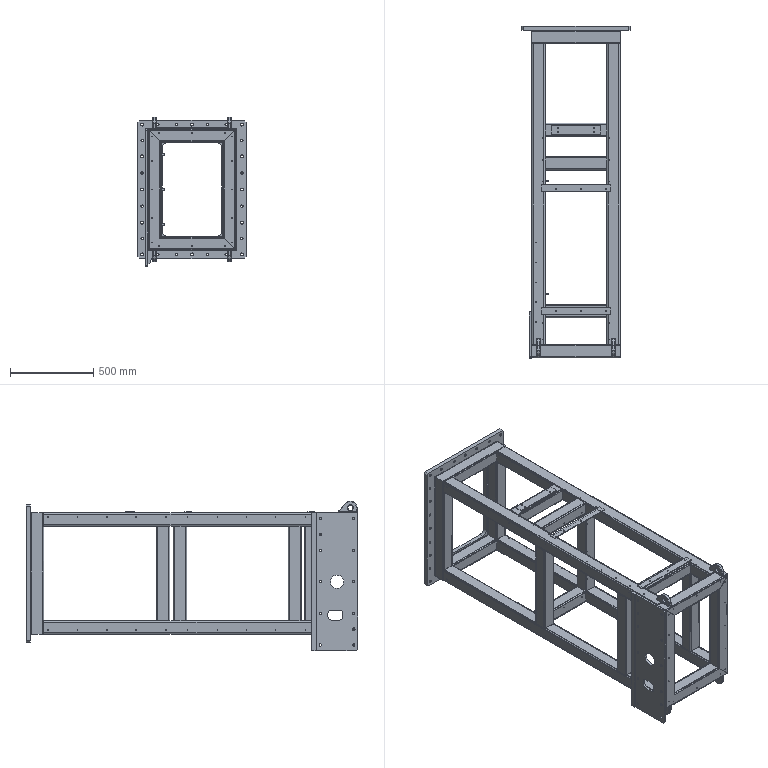Part | SolidWorks | 33 solids | 941 faces | box 650 x 1995 x 900 mm | volume 30095229 mm3 | cylinder 595 | plane 298 | torus 24 | cone 16 | sphere 8 | commonest cylinder face diameters 3.3 x238 8 x92 16 x84 14 x54 6 x28 6.8 x26